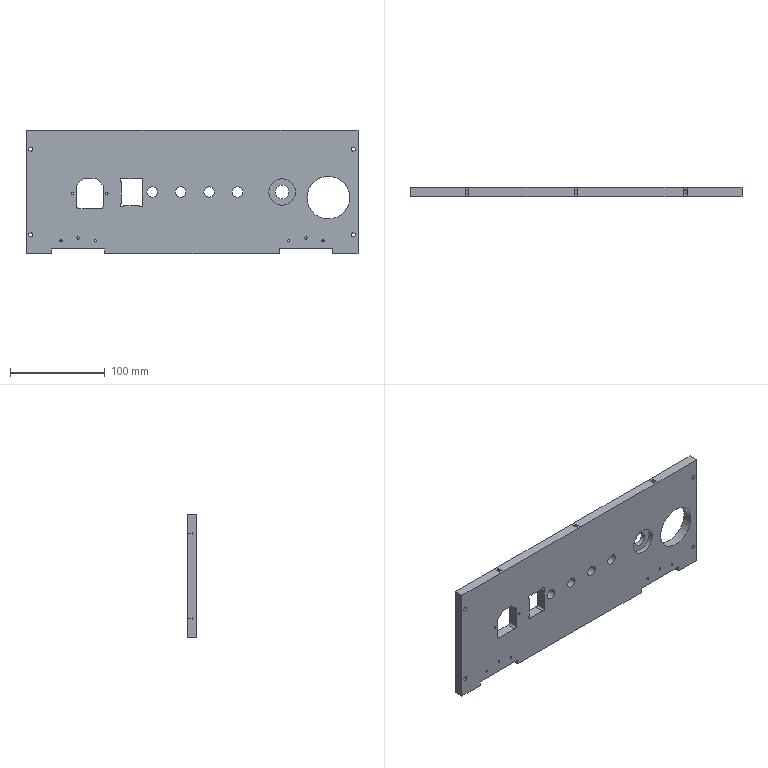Part | SolidWorks | features BaseBody 1 | 1 solid | 104 faces | box 350 x 10 x 130 mm | volume 408343 mm3 | cylinder 69 | plane 35 | commonest cylinder face diameters 2.5 x16 4.2 x11 8 x8 11 x8 3.3 x6 4 x6